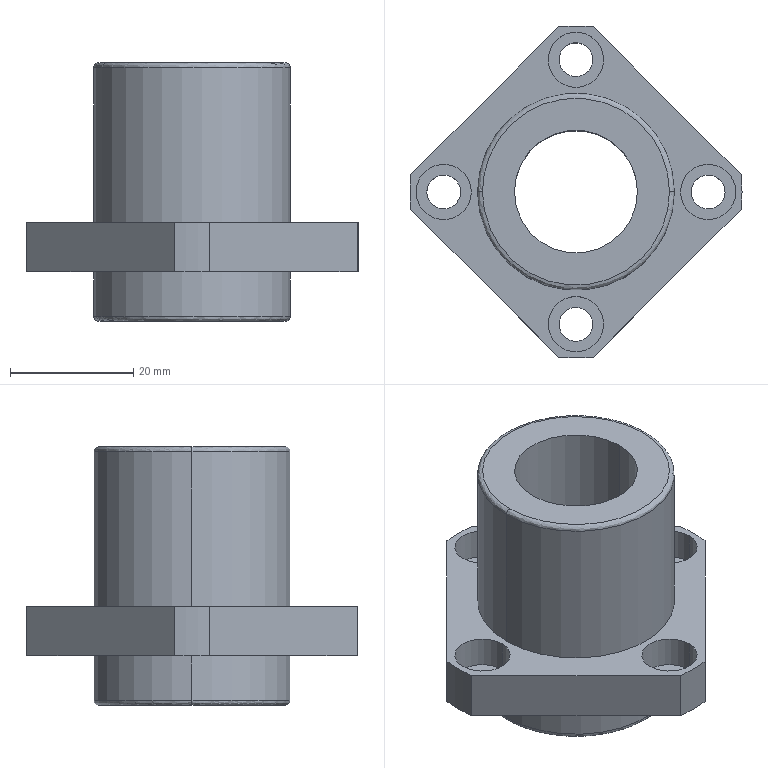Part | STEP file | Flanged linear bearing LMJ11-D20 | 1 solid | 43 faces | box 54 x 54 x 42 mm | volume 26412 mm3 | cylinder 27 | plane 12 | spline 4 | commonest cylinder face diameters 5.5 x8 9 x8 54 x5 32 x4 20 x2